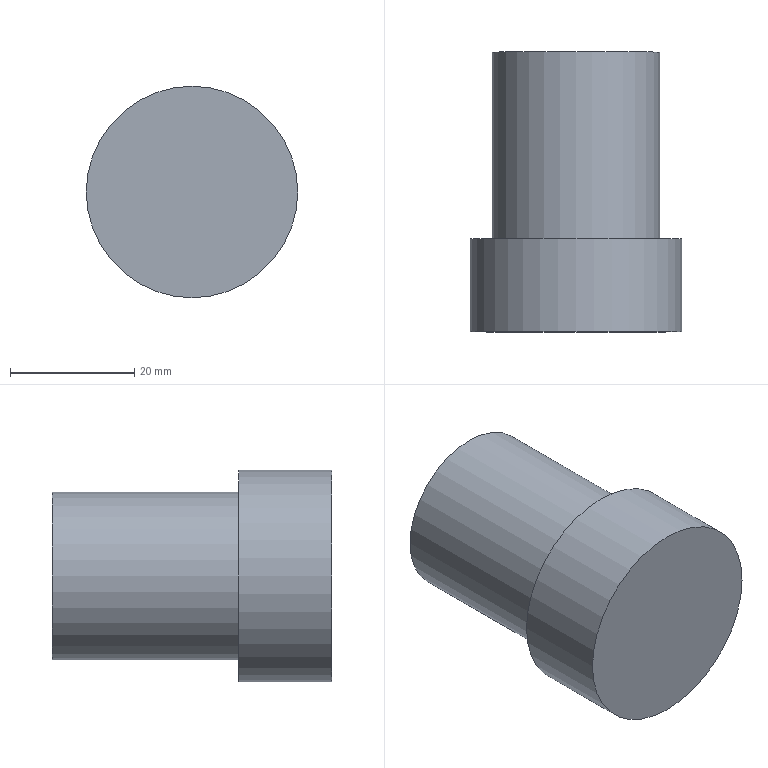Part | NX | features solid 2 | 1 solid | 5 faces | box 34 x 45 x 34 mm | volume 30795 mm3 | plane 3 | cylinder 2 | commonest cylinder face diameters 27 x1 34 x1
STEP:
#1=CARTESIAN_POINT('',(420.,430.,-347.));
#2=VERTEX_POINT('',#1);
#3=CARTESIAN_POINT('',(420.,430.,-330.));
#4=DIRECTION('',(0.,1.,0.));
#5=DIRECTION('',(0.,0.,-1.));
#6=AXIS2_PLACEMENT_3D('',#3,#4,#5);
#7=CIRCLE('',#6,17.);
#8=EDGE_CURVE('',#2,#2,#7,.T.);
#9=ORIENTED_EDGE('',*,*,#8,.T.);
#10=EDGE_LOOP('',(#9));
#11=FACE_BOUND('',#10,.T.);
#12=CARTESIAN_POINT('',(420.,430.,-343.5));
#13=VERTEX_POINT('',#12);
#14=CARTESIAN_POINT('',(420.,430.,-330.));
#15=DIRECTION('',(0.,1.,0.));
#16=DIRECTION('',(0.,0.,-1.));
#17=AXIS2_PLACEMENT_3D('',#14,#15,#16);
#18=CIRCLE('',#17,13.5);
#19=EDGE_CURVE('',#13,#13,#18,.F.);
#20=ORIENTED_EDGE('',*,*,#19,.T.);
#21=EDGE_LOOP('',(#20));
#22=FACE_BOUND('',#21,.T.);
#23=CARTESIAN_POINT('',(420.,430.,-316.5));
#24=DIRECTION('',(0.,-1.,0.));
#25=DIRECTION('',(0.,0.,-1.));
#26=AXIS2_PLACEMENT_3D('',#23,#24,#25);
#27=PLANE('',#26);
#28=ADVANCED_FACE('',(#11,#22),#27,.F.);
#29=CARTESIAN_POINT('',(420.,415.,-347.));
#30=VERTEX_POINT('',#29);
#31=CARTESIAN_POINT('',(420.,415.,-330.));
#32=DIRECTION('',(0.,1.,0.));
#33=DIRECTION('',(0.,0.,-1.));
#34=AXIS2_PLACEMENT_3D('',#31,#32,#33);
#35=CIRCLE('',#34,17.);
#36=EDGE_CURVE('',#30,#30,#35,.T.);
#37=ORIENTED_EDGE('',*,*,#36,.T.);
#38=EDGE_LOOP('',(#37));
#39=FACE_BOUND('',#38,.T.);
#40=ORIENTED_EDGE('',*,*,#8,.F.);
#41=EDGE_LOOP('',(#40));
#42=FACE_BOUND('',#41,.T.);
#43=CARTESIAN_POINT('',(420.,415.,-330.));
#44=DIRECTION('',(0.,1.,0.));
#45=DIRECTION('',(0.,0.,1.));
#46=AXIS2_PLACEMENT_3D('',#43,#44,#45);
#47=CYLINDRICAL_SURFACE('',#46,17.);
#48=ADVANCED_FACE('',(#39,#42),#47,.T.);
#49=ORIENTED_EDGE('',*,*,#36,.F.);
#50=EDGE_LOOP('',(#49));
#51=FACE_BOUND('',#50,.T.);
#52=CARTESIAN_POINT('',(420.,415.,-316.5));
#53=DIRECTION('',(0.,-1.,0.));
#54=DIRECTION('',(0.,0.,-1.));
#55=AXIS2_PLACEMENT_3D('',#52,#53,#54);
#56=PLANE('',#55);
#57=ADVANCED_FACE('',(#51),#56,.T.);
#58=CARTESIAN_POINT('',(420.,460.,-343.5));
#59=VERTEX_POINT('',#58);
#60=CARTESIAN_POINT('',(420.,460.,-330.));
#61=DIRECTION('',(0.,1.,0.));
#62=DIRECTION('',(0.,0.,-1.));
#63=AXIS2_PLACEMENT_3D('',#60,#61,#62);
#64=CIRCLE('',#63,13.5);
#65=EDGE_CURVE('',#59,#59,#64,.T.);
#66=ORIENTED_EDGE('',*,*,#65,.F.);
#67=EDGE_LOOP('',(#66));
#68=FACE_BOUND('',#67,.T.);
#69=ORIENTED_EDGE('',*,*,#19,.F.);
#70=EDGE_LOOP('',(#69));
#71=FACE_BOUND('',#70,.T.);
#72=CARTESIAN_POINT('',(420.,460.,-330.));
#73=DIRECTION('',(0.,-1.,0.));
#74=DIRECTION('',(0.,0.,-1.));
#75=AXIS2_PLACEMENT_3D('',#72,#73,#74);
#76=CYLINDRICAL_SURFACE('',#75,13.5);
#77=ADVANCED_FACE('',(#68,#71),#76,.T.);
#78=ORIENTED_EDGE('',*,*,#65,.T.);
#79=EDGE_LOOP('',(#78));
#80=FACE_BOUND('',#79,.T.);
#81=CARTESIAN_POINT('',(420.,460.,-316.5));
#82=DIRECTION('',(0.,-1.,0.));
#83=DIRECTION('',(0.,0.,-1.));
#84=AXIS2_PLACEMENT_3D('',#81,#82,#83);
#85=PLANE('',#84);
#86=ADVANCED_FACE('',(#80),#85,.F.);
#87=CLOSED_SHELL('',(#28,#48,#57,#77,#86));
#88=MANIFOLD_SOLID_BREP('',#87);
#89=(LENGTH_UNIT()NAMED_UNIT(*)SI_UNIT(.MILLI.,.METRE.));
#90=UNCERTAINTY_MEASURE_WITH_UNIT(LENGTH_MEASURE(0.00001),#89,'','');
#91=(NAMED_UNIT(*)PLANE_ANGLE_UNIT()SI_UNIT($,.RADIAN.));
#92=(NAMED_UNIT(*)SI_UNIT($,.STERADIAN.)SOLID_ANGLE_UNIT());
#93=(GEOMETRIC_REPRESENTATION_CONTEXT(3)GLOBAL_UNCERTAINTY_ASSIGNED_CONTEXT((#90))GLOBAL_UNIT_ASSIGNED_CONTEXT((#89,#91,#92))REPRESENTATION_CONTEXT('',''));
#94=ADVANCED_BREP_SHAPE_REPRESENTATION('',(#88),#93);